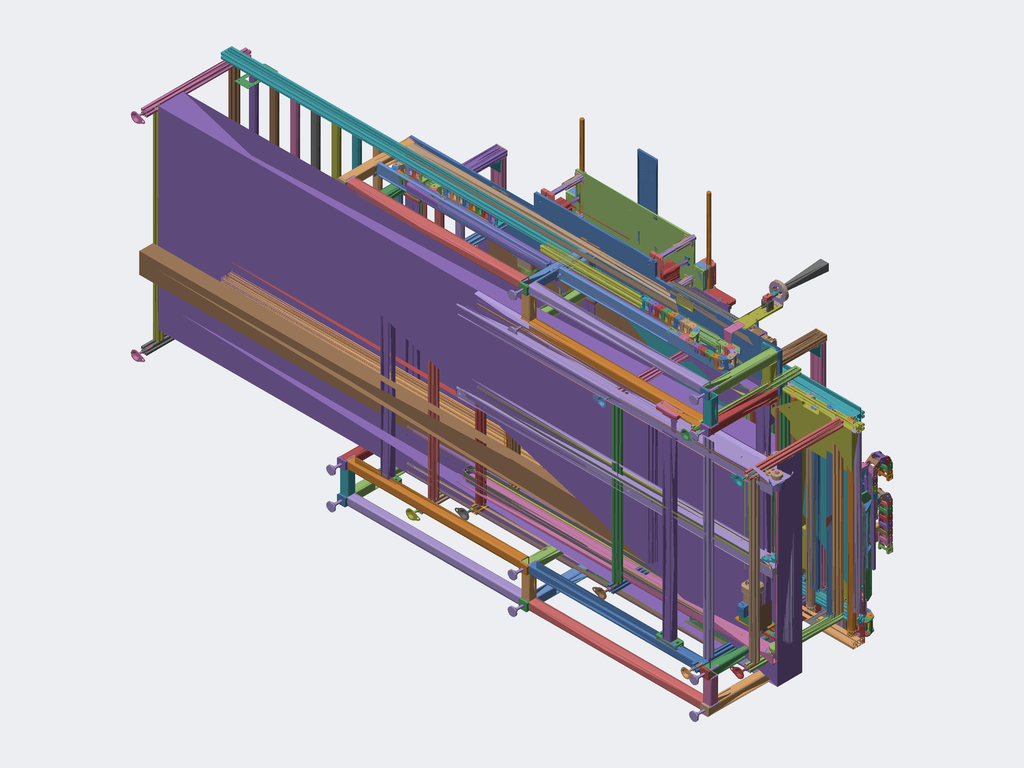Assembly | SolidWorks | 202 different items | 963 placed
Parts list (item | name | quantity | parent item | size | volume | features):
1 | (subassembly) | x2 | in 4 | 57 x 22 x 94 mm | 6979 mm3 | -
2 | (subassembly) | x1 | - | 145.001 x 61.5 x 34.5 mm | 436021 mm3 | -
3 | (subassembly) | x1 | - | 83.2 x 24 x 135 mm | 27538 mm3 | -
4 | (subassembly) | x2 | - | 64 x 60 x 671 mm | 1247970 mm3 | -
5 | (subassembly) | x2 | in 15 | 1463 x 40 x 40 mm | 130548 mm3 | -
6 | (subassembly) | x5 | in 13 | - | 74187256 mm3 | features ReferencePattern 34, LocalLPattern 3
7 | (subassembly) | x21 | in 18 | 95.3 x 80 x 116.633 mm | 320857 mm3 | -
8 | (subassembly) | x2 | - | 223.5 x 705 x 120 mm | 1273117 mm3 | features CompositeCurve 1
9 | (subassembly) | x2 | in 21, 22 | 142.5 x 477.965 x 120 mm | 1151142 mm3 | features ReferencePattern 6, InContextFeatHolder 2, CompositeCurve 1, LocalLPattern 1
10 | (subassembly) | x4 | in 19, 20 | 204 x 77 x 84 mm | 434745 mm3 | -
11 | (subassembly) | x20 | in 14, 16 | 30 x 39 x 30 mm | 17492 mm3 | -
12 | (subassembly) | x1 | - | - | 88653077 mm3 | features ReferencePattern 7, MirrorCompFeat 2, DerivedHolePattern 1
13 | (subassembly) | x1 | - | - | - | features ReferencePattern 40, LocalLPattern 5
14 | (subassembly) | x2 | in 19, 20 | 1270 x 60 x 664 mm | 3435142 mm3 | features ReferencePattern 7, DerivedHolePattern 1, MirrorCompFeat 1
15 | (subassembly) | x2 | - | - | 11809484 mm3 | -
16 | (subassembly) | x2 | in 15 | 190 x 410 x 1645 mm | 3631798 mm3 | features ReferencePattern 6, DerivedHolePattern 1, MirrorCompFeat 1
17 | (subassembly) | x1 | - | - | - | features ReferencePattern 3, CompositeCurve 2, DerivedHolePattern 1
18 | (subassembly) | x7 | in 6, 13 | 1198 x 199.551 x 2300 mm | 9436747 mm3 | features InContextFeatHolder 2, MirrorCompFeat 1, ReferencePattern 1
19 | (subassembly) | x1 | in 12 | - | 39858660 mm3 | features ReferencePattern 11, DerivedHolePattern 2, CompositeCurve 1
20 | (subassembly) | x1 | in 12 | - | 41125199 mm3 | features ReferencePattern 11, DerivedHolePattern 2, CompositeCurve 1
21 | (subassembly) | x1 | in 17 | - | 8582117 mm3 | features ReferencePattern 2, LocalLPattern 1
22 | (subassembly) | x1 | in 17 | - | - | features ReferencePattern 2, CompositeCurve 1, LocalLPattern 1
23 | (subassembly) | x2 | in 17 | 34 x 24 x 680 mm | 137302 mm3 | -
24 | (subassembly) | x2 | in 15 | - | 9829860 mm3 | -
25 | (subassembly) | x2 | in 24 | 123 x 66.8 x 864 mm | 3505638 mm3 | -
26 | (subassembly) | x2 | in 24 | 236 x 83 x 1039 mm | 3946589 mm3 | -
27 | (subassembly) | x2 | in 26 | 172 x 64 x 60 mm | 126138 mm3 | -
28 | Bearing_6004_D42Xd20XT12_Deep Groove Ball Bearing[GBT276-94 | x1 | - | - | - | -
29 | - | x6 | in 8, 9 | 29 x 29.002 x 60.3 mm | 34730 mm3 | features BaseBody 3
30 | - | x7 | in 18 | 282.879 x 60 x 52 mm | 48298 mm3 | features ICE 8, Fillet 3, Extrusion 1, FlatPattern 1, FlattenBends 1, ProcessBends 1, Rip 1, SheetMetal 1, Shell 1
31 | - | x12 | in 6, 13 | 2 x 220 x 100 mm | 34889 mm3 | features ExtruThin 1, Fillet 1, ICE 1
32 | - | x21 | in 7 | 80 x 80 x 50 mm | 223390 mm3 | features ICE 2, CirPattern 1, Extrusion 1, HoleWzd 1, RevCut 1
33 | - | x7 | in 18 | 20 x 20 x 1198 mm | 373288 mm3 | features Extrusion 1, ICE 1
34 | - | x7 | in 18 | 24.001 x 54.65 x 54.65 mm | 18054 mm3 | features BaseBody 1, CirPattern 1, HoleWzd 1
35 | - | x7 | in 18 | 24.001 x 54.65 x 54.65 mm | 19561 mm3 | features BaseBody 1, HoleWzd 1, ICE 1
36 | - | x80 | in 6 | 50 x 50 x 1170 mm | 2265436 mm3 | features HoleWzd 2, ICE 2, Chamfer 1, Extrusion 1, MirrorPattern 1, RevCut 1
37 | - | x6 | in 6, 13 | 43 x 43 x 30 mm | 35397 mm3 | features Extrusion 1, ICE 1
38 | - | x5 | in 6 | 1250 x 740 x 2300 mm | 23808446 mm3 | features ICE 4, Extrusion 1, HoleWzd 1, LPattern 1
39 | - | x2 | in 21, 22 | 630 x 15 x 85 mm | 135946 mm3 | features HoleWzd 3, EdgeFlange 1, Fillet 1, FlatPattern 1, SMBaseFlange 1, SheetMetal 1
40 | - | x8 | in 10 | 40.5 x 5.8 x 4.4 mm | 628.814 mm3 | features BaseBody 1
41 | - | x2 | in 17 | 430 x 20 x 115 mm | 126667 mm3 | features HoleWzd 4, EdgeFlange 1, Fillet 1, FlatPattern 1, SMBaseFlange 1, SheetMetal 1
42 | - | x2 | - | 1259 x 38 x 85 mm | 278401 mm3 | features HoleWzd 4, EdgeFlange 2, Fillet 1, FlatPattern 1, SMBaseFlange 1, SheetMetal 1
43 | - | x4 | in 8, 9 | 100 x 100 x 55 mm | 20982 mm3 | features HoleWzd 3, Fillet 1, FlatPattern 1, SMBaseFlange 1, SheetMetal 1
44 | - | x2 | in 17, 22 | 107.5 x 30 x 55 mm | 14107 mm3 | features HoleWzd 3, Fillet 1, FlatPattern 1, SMBaseFlange 1, SheetMetal 1
45 | - | x6 | in 8, 9 | 125.5 x 22 x 120 mm | 19406 mm3 | features HoleWzd 2, ICE 2, Fillet 1, FlatPattern 1, SMBaseFlange 1, SheetMetal 1
46 | - | x4 | in 9 | 45 x 51 x 60 mm | 15618 mm3 | features ICE 2, ExtruThin 1, Fillet 1, FlatPattern 1, FlattenBends 1, ProcessBends 1, SheetMetal 1
47 | - | x2 | in 15 | 120 x 30 x 360 mm | 79726 mm3 | features ExtruThin 1, Fillet 1, FlatPattern 1, FlattenBends 1, ICE 1, ProcessBends 1, SheetMetal 1
48 | - | x2 | in 15 | 90 x 50 x 80 mm | 23252 mm3 | features ICE 3, ExtruThin 1, Fillet 1
49 | - | x2 | in 9 | 90 x 250 x 5 mm | 108732 mm3 | features ICE 3, Extrusion 1, Fillet 1
50 | - | x4 | in 16 | 190 x 15 x 70 mm | 186782 mm3 | features HoleWzd 4, Chamfer 1, Extrusion 1
51 | - | x12 | in 19, 20 | 60 x 179 x 60 mm | 83421 mm3 | features BaseBody 2
52 | - | x2 | in 16 | 10 x 115 x 370 mm | 331477 mm3 | features HoleWzd 2, Chamfer 1, Extrusion 1, ICE 1
53 | - | x2 | in 16 | 65 x 12 x 370 mm | 282662 mm3 | features HoleWzd 2, Chamfer 1, Extrusion 1, LPattern 1
54 | - | x2 | in 21, 22 | 12 x 105 x 690 mm | 852566 mm3 | features HoleWzd 4, Chamfer 2, Extrusion 1
55 | - | x1 | in 22 | 145 x 12 x 690 mm | 673672 mm3 | features HoleWzd 6, Chamfer 2, Extrusion 1, ICE 1
56 | - | x2 | in 9 | 100 x 148 x 12 mm | 172636 mm3 | features HoleWzd 6, Extrusion 1
57 | - | x2 | in 8 | 80 x 285 x 12 mm | 259377 mm3 | features HoleWzd 5, Chamfer 1, Extrusion 1, ICE 1
58 | - | x4 | in 8, 9 | 50 x 42 x 55 mm | 47186 mm3 | features HoleWzd 2, ICE 2, Chamfer 1, Extrusion 1
59 | - | x1 | in 21 | 145 x 12 x 690 mm | 673672 mm3 | features MirrorStock 1
60 | - | x6 | in 21, 22 | 58 x 10 x 95 mm | 33990 mm3 | features HoleWzd 2, Extrusion 1, ICE 1
61 | - | x4 | in 12 | 130 x 30.7 x 50 mm | 191359 mm3 | features HoleWzd 2, Chamfer 1, Extrusion 1
62 | - | x2 | in 23 | 15 x 12.5 x 680 mm | 106806 mm3 | features ICE 2, BaseBody 1, HoleWzd 1
63 | - | x2 | in 8 | 75 x 10 x 80 mm | 56721 mm3 | features HoleWzd 3, Chamfer 1, Extrusion 1
64 | - | x2 | in 8 | 75 x 10 x 120 mm | 34697 mm3 | features Fillet 2, HoleWzd 2, Extrusion 1, ICE 1
65 | - | x2 | in 21, 22 | 55 x 12 x 148 mm | 94373 mm3 | features HoleWzd 3, Chamfer 1, Extrusion 1
66 | - | x2 | in 21, 22 | 110 x 10 x 105 mm | 47398 mm3 | features Chamfer 1, Extrusion 1, HoleWzd 1, ICE 1, MirrorPattern 1
67 | - | x4 | in 17 | 15 x 13 x 10 mm | 1585 mm3 | features Extrusion 1, HoleWzd 1
68 | - | x4 | in 19, 20 | 310 x 20 x 80 mm | 438735 mm3 | features HoleWzd 4, ICE 2, Chamfer 1, Extrusion 1
69 | - | x4 | in 14 | 15 x 26 x 40 mm | 14020 mm3 | features Chamfer 2, HoleWzd 2, Extrusion 1
70 | - | x2 | in 19, 20 | 1000 x 12 x 320 mm | 3431289 mm3 | features HoleWzd 5, Chamfer 1, Extrusion 1, ICE 1
71 | - | x4 | in 19, 20 | 76 x 41.5 x 130 mm | 406429 mm3 | features Chamfer 1, Extrusion 1, HoleWzd 1
72 | - | x2 | in 14 | 135 x 605 x 12 mm | 965539 mm3 | features HoleWzd 3, Extrusion 1
73 | - | x2 | in 23 | 34 x 19.5 x 57.8 mm | 30496 mm3 | features BaseBody 1
74 | - | x2 | in 14 | 1270 x 60 x 12 mm | 902865 mm3 | features HoleWzd 4, Chamfer 1, Extrusion 1
75 | - | x2 | in 14 | 1270 x 12 x 47 mm | 615944 mm3 | features HoleWzd 4, ICE 2, Chamfer 1, Extrusion 1
76 | - | x8 | in 14 | 25 x 10 x 40 mm | 4716 mm3 | features HoleWzd 2, Chamfer 1, Extrusion 1, ICE 1
77 | - | x2 | in 14 | 1270 x 6 x 15 mm | 113647 mm3 | features Chamfer 1, Extrusion 1, HoleWzd 1
78 | - | x1 | in 20 | 2700 x 15 x 390 mm | 12856560 mm3 | features HoleWzd 7, ICE 4, Chamfer 1, Extrusion 1, Fillet 1, PLine 1
79 | - | x1 | in 19 | 2700 x 15 x 330 mm | 12065498 mm3 | features HoleWzd 7, ICE 4, Chamfer 1, Extrusion 1, Fillet 1, PLine 1
80 | - | x2 | in 16 | 370 x 80 x 1615 mm | 2239494 mm3 | features WeldCornerFeat 2, WeldMemberFeat 2, WeldmentFeature 1
81 | - | x2 | in 19, 20 | 2700 x 516 x 300 mm | 16210960 mm3 | features HoleWzd 9, WeldCornerFeat 6, ICE 4, WeldMemberFeat 3, 3DProfileFeature 1, WeldmentFeature 1
82 | - | x5 | in 12 | 1451 x 150 x 60 mm | 1723034 mm3 | features HoleWzd 2, ICE 1, MirrorSolid 1, WeldMemberFeat 1, WeldmentFeature 1
83 | - | x4 | in 14 | 70 x 70 x 36 mm | 47267 mm3 | features BaseBody 2
84 | - | x1 | in 17 | 129.5 x 557 x 2700 mm | 6948408 mm3 | features HoleWzd 6, ICE 6, Chamfer 3, MirrorSolid 3, WeldMemberFeat 2, MirrorPattern 1, WeldCornerFeat 1, WeldmentFeature 1
85 | - | x4 | in 5 | 66 x 40 x 40 mm | 65274 mm3 | features BaseBody 3
86 | - | x6 | in 8, 9 | 120 x 120 x 20 mm | 177458 mm3 | features Chamfer 1, Extrusion 1, ICE 1
87 | - | x63 | in 7 | 28 x 13 x 13 mm | 1916 mm3 | features BaseBody 1
88 | - | x4 | in 24 | 42.996 x 43 x 52 mm | 57062 mm3 | features BaseBody 1
89 | - | x31 | in 13 | 1380 x 51.459 x 51.986 mm | 596958 mm3 | features ICE 6, BaseBody 1, HoleWzd 1, LPattern 1
90 | - | x1 | in 13 | 1540 x 775 x 4600 mm | 1226148521 mm3 | features ICE 4, BossThin 1, Extrusion 1, LPattern 1
91 | - | x1 | in 13 | 2100 x 85 x 1250 mm | 164068651 mm3 | features ICE 3, BaseBody 1
92 | - | x36 | in 6, 13 | 68 x 121 x 100 mm | 26277 mm3 | features BaseBody 2
93 | - | x1 | - | - | - | features BaseBody 181
94 | - | x2 | in 17 | 912 x 76 x 178.533 mm | 5760586 mm3 | features BaseBody 18, LPattern 1
95 | - | x2 | in 24 | 20 x 20 x 1414 mm | 444221 mm3 | features BaseBody 1, ICE 1
96 | - | x6 | in 8, 9 | 60 x 50 x 350 mm | 603883 mm3 | features Blend 1, Cut 1
97 | - | x6 | in 6, 13 | 60 x 102 x 102.7 mm | 330811 mm3 | features BaseBody 1
98 | - | x7 | in 18 | 189.793 x 59.207 x 17 mm | 45007 mm3 | features ICE 6, Extrusion 1, MirrorPattern 1
99 | - | x4 | in 14 | 25 x 25 x 605 mm | 295385 mm3 | features HoleWzd 2, Chamfer 1, Extrusion 1
100 | - | x8 | in 19, 20 | 30 x 320 x 30 mm | 223294 mm3 | features HoleWzd 2, Chamfer 1, Extrusion 1
101 | - | x7 | in 18 | 72.5 x 159.151 x 2300 mm | 2459772 mm3 | features MirrorStock 1
102 | - | x6 | in 8, 9 | 28 x 34 x 34 mm | 18676 mm3 | features BaseBody 1
103 | - | x1 | in 13 | 57 x 40 x 4600 mm | 1199908 mm3 | features FlatPattern 1, SMBaseFlange 1, SheetMetal 1
104 | - | x21 | in 18 | 2303 x 86 x 50 mm | 856015 mm3 | features ExtruThin 1, Sweep 1
105 | - | x2 | in 21, 22 | 846 x 78 x 155.983 mm | 3838059 mm3 | features BaseBody 19
106 | - | x8 | in 19, 20 | 74 x 74 x 123 mm | 122760 mm3 | features BaseBody 1
107 | - | x4 | in 19, 20 | 76 x 51.5 x 130 mm | 357296 mm3 | features BaseBody 1
108 | - | x13 | in 6, 13, 18 | 273 x 143.386 x 105.972 mm | 1078601 mm3 | features BaseBody 4
109 | - | x16 | in 25, 26 | 24.5 x 15.5 x 50 mm | 13570 mm3 | features BaseBody 1
110 | - | x2 | in 26 | 8.5 x 35.5 x 30 mm | 877.993 mm3 | features BaseBody 1
111 | - | x2 | in 27 | 172 x 64 x 46 mm | 45275 mm3 | features BaseBody 1
112 | - | x2 | in 27 | 172 x 64 x 14 mm | 80863 mm3 | features BaseBody 1
113 | - | x4 | in 25, 26 | 65 x 66.1 x 67 mm | 277180 mm3 | features BaseBody 3
114 | - | x4 | in 24 | 63 x 18.5 x 246 mm | 256185 mm3 | features BaseBody 1
115 | - | x2 | in 25 | 105.5 x 66.1 x 77 mm | 335496 mm3 | features BaseBody 2
116 | - | x2 | in 26 | 142 x 66.1 x 77 mm | 347121 mm3 | features BaseBody 2
117 | - | x4 | in 25, 26 | 65 x 65 x 720 mm | 2838677 mm3 | features BaseBody 1
118 | - | x8 | in 15, 17, 19, 20, 21, 22 | - | - | features RefSurface 65
119 | - | x4 | in 16 | 40 x 5 x 80 mm | 15913 mm3 | features Extrusion 1, Fillet 1
120 | - | x2 | in 26 | - | - | features RefSurface 10
121 | - | x2 | in 4 | 54 x 50 x 604 mm | 1228026 mm3 | features BaseBody 1
122 | - | x2 | in 4 | 32 x 7.6 x 48 mm | 3951 mm3 | features BaseBody 1
123 | - | x2 | in 4 | 53 x 57 x 13 mm | 21853 mm3 | features BaseBody 1
124 | - | x2 | in 4 | 53 x 56.359 x 48 mm | 87261 mm3 | features BaseBody 1
125 | - | x2 | in 1 | 12 x 16.25 x 5.5 mm | 322.658 mm3 | features BaseBody 1
126 | - | x2 | in 4 | 27 x 18 x 18 mm | 1018 mm3 | features BaseBody 1
127 | - | x2 | in 1 | 5.54 x 2 x 5.54 mm | 44.4 mm3 | features BaseBody 1
128 | - | x2 | in 1 | 5.54 x 2 x 5.54 mm | 44.4 mm3 | features BaseBody 1
129 | - | x2 | in 1 | 5.54 x 2 x 5.54 mm | 44.4 mm3 | features BaseBody 1
130 | - | x1 | - | 2060 x 50 x 1250 mm | 5816564 mm3 | features ICE 5, Extrusion 1
131 | - | x2 | in 1 | 5.54 x 2 x 5.54 mm | 44.4 mm3 | features BaseBody 1
132 | - | x2 | in 1 | - | - | features RefSurface 1
133 | - | x2 | in 1 | - | - | features RefSurface 1
134 | - | x2 | in 1 | - | - | features RefSurface 1
135 | - | x2 | in 1 | - | - | features RefSurface 1
136 | - | x2 | in 4 | - | - | features RefSurface 2
137 | - | x2 | in 4 | 54 x 47.5 x 10 mm | 14283 mm3 | features BaseBody 1
138 | - | x2 | in 4 | 13.6 x 15.5 x 27.7 mm | 2180 mm3 | features BaseBody 1
139 | - | x2 | in 4 | 27 x 18 x 18 mm | 1018 mm3 | features BaseBody 1
140 | - | x2 | in 4 | 13.6 x 15.5 x 27.7 mm | 2180 mm3 | features BaseBody 1
141 | - | x6 | in 26 | 26 x 39 x 13.7 mm | 3551 mm3 | features BaseBody 1
142 | - | x2 | in 4 | 13.6 x 15.5 x 27.7 mm | 2180 mm3 | features BaseBody 1
143 | - | x2 | in 4 | 27 x 18 x 18 mm | 1018 mm3 | features BaseBody 1
144 | - | x1 | - | 82 x 66 x 554 mm | 2405342 mm3 | features BaseBody 1
145 | - | x1 | - | 13.6 x 15.5 x 27.7 mm | 2180 mm3 | features BaseBody 1
146 | - | x1 | - | 13.6 x 15.5 x 27.7 mm | 2180 mm3 | features BaseBody 1
147 | - | x1 | - | 27 x 18 x 18 mm | 1018 mm3 | features BaseBody 1
148 | - | x1 | - | 13.6 x 15.5 x 27.7 mm | 2180 mm3 | features BaseBody 1
149 | - | x1 | - | 146 x 62 x 12 mm | 64829 mm3 | features BaseBody 1
150 | - | x1 | - | 140.075 x 56.575 x 22.3 mm | 156798 mm3 | features BaseBody 1
151 | - | x1 | - | - | - | features RefSurface 1
152 | - | x4 | in 16 | 80.8 x 80.8 x 76 mm | 99581 mm3 | features BaseBody 1
153 | - | x1 | - | - | - | features RefSurface 1
154 | - | x1 | - | - | - | features RefSurface 1
155 | - | x1 | - | - | - | features RefSurface 1
156 | - | x1 | - | - | - | features RefSurface 1
157 | - | x1 | - | 5.5 x 5.5 x 3 mm | 63.35 mm3 | features BaseBody 1
158 | - | x1 | - | 5.5 x 5.5 x 3 mm | 63.35 mm3 | features BaseBody 1
159 | - | x1 | - | 5.5 x 5.5 x 3 mm | 63.35 mm3 | features BaseBody 1
160 | - | x1 | - | 5.5 x 5.5 x 3 mm | 63.35 mm3 | features BaseBody 1
161 | - | x1 | - | 145.001 x 61.5 x 34.5 mm | 279097 mm3 | features BaseBody 1
162 | - | x1 | - | - | - | features RefSurface 1
163 | - | x4 | in 16 | 80 x 80 x 30 mm | 51823 mm3 | features BaseBody 1
164 | - | x1 | - | - | - | features RefSurface 1
165 | - | x1 | - | - | - | features RefSurface 1
166 | - | x1 | - | 5.54 x 2 x 5.54 mm | 44.4 mm3 | features BaseBody 1
167 | - | x1 | - | 5.54 x 2 x 5.54 mm | 44.4 mm3 | features BaseBody 1
168 | - | x1 | - | 5.54 x 2 x 5.54 mm | 44.4 mm3 | features BaseBody 1
169 | - | x1 | - | 5.54 x 2 x 5.54 mm | 44.4 mm3 | features BaseBody 1
170 | - | x1 | - | - | - | features RefSurface 1
171 | - | x1 | - | - | - | features RefSurface 1
172 | - | x1 | - | - | - | features RefSurface 1
173 | - | x1 | - | - | - | features RefSurface 1
174 | - | x4 | in 10 | 121 x 84 x 77 mm | 331799 mm3 | features BaseBody 1
175 | - | x1 | - | 80 x 63 x 15 mm | 53710 mm3 | features BaseBody 1
176 | - | x1 | - | 82 x 73.6 x 37.1 mm | 61964 mm3 | features BaseBody 1
177 | - | x1 | - | 4 x 17 x 15 mm | 361.162 mm3 | features BaseBody 1
178 | - | x1 | - | 27 x 18 x 18 mm | 1018 mm3 | features BaseBody 1
179 | - | x1 | - | 27 x 18 x 18 mm | 1018 mm3 | features BaseBody 1
180 | - | x80 | in 6 | 195.3 x 45.3 x 7 mm | 6104 mm3 | features ExtruThin 1
181 | - | x5 | in 6 | 195.3 x 45.3 x 9.4 mm | 8197 mm3 | features ExtruThin 1
182 | - | x20 | in 11 | 30 x 30 x 39 mm | 17492 mm3 | features BaseBody 1, ICE 1
183 | - | x2 | in 26 | 116 x 65 x 65 mm | 248255 mm3 | features BaseBody 3
184 | - | x2 | in 15 | 165 x 64 x 30 mm | 211731 mm3 | features BaseBody 2
185 | - | x4 | in 10 | 121.5 x 62.5 x 62.5 mm | 101686 mm3 | features BaseBody 1
186 | - | x21 | in 7 | 110 x 62 x 33.3 mm | 91720 mm3 | features ICE 2, Extrusion 1
187 | - | x4 | in 24 | 127 x 65 x 38 mm | 109407 mm3 | features BaseBody 1
188 | - | x2 | in 21, 22 | - | 832857 mm3 | features BaseBody 13, LPattern 4
189 | - | x2 | - | - | 907035 mm3 | features BaseBody 13, LPattern 3
190 | - | x2 | in 17 | - | 1022357 mm3 | features BaseBody 13, LPattern 3
191 | - | x4 | in 19, 20 | 36 x 52 x 24 mm | 16208 mm3 | features BaseBody 2, Chamfer 1, ICE 1
192 | - | x6 | in 6, 13 | 90 x 203 x 135 mm | 261739 mm3 | features ICE 2, ExtruThin 1, Fillet 1
193 | - | x7 | in 18 | 72.5 x 159.151 x 2300 mm | 2459772 mm3 | features ICE 6, BossThin 2, Fillet 2, ExtruThin 1, FlatPattern 1, FlattenBends 1, ProcessBends 1, SheetMetal 1
194 | - | x7 | in 18 | 60 x 108 x 2300 mm | 1846867 mm3 | features ICE 6, Fillet 3, BossThin 2, ExtruThin 1, FlatPattern 1, FlattenBends 1, ProcessBends 1, SheetMetal 1
195 | - | x7 | in 18 | 140 x 113 x 190 mm | 218037 mm3 | features ICE 6, Fillet 3, Cut 1, DeleteBody 1, ExtruThin 1, MirrorSolid 1
196 | - | x1 | - | - | - | features RefSurface 137, BaseBody 102
197 | GRH8-L10-400-BL-P40-C4_0 | x1 | - | - | - | -
198 | MKR65-R-X1 (subassembly) | x1 | - | - | - | -
199 | MKR65-X2 (subassembly) | x1 | - | - | - | -
200 | SJCB- 40C- RD_SJCB-40C-16X18 | x1 | - | - | - | -
201 | 同动轴 | x1 | - | - | - | -
202 | 轴承支撑座 | x1 | - | - | - | -
Mates (type | each side: item.copy, entity, surface, feature):
In the top assembly
Coincident | assembly face | assembly face
Slot | assembly face | assembly face | 2 times
Coincident | 77.1 face plane Boss-Extrude 1 | 130.1 face plane Boss-Extrude 1
Coincident | 79.1 face plane 分割线1 | 84.1 face plane Boss-Extrude 2
Concentric | 79.1 face cylinder M8 Tapped Hole 2 | 84.1 face cylinder Ø9.0 (9) DiameterHole 1 | 2 times
Slot | 79.1 face cylinder M5 Tapped Hole 1 | 109.1 face plane 输入1
Coincident | 78.1 face plane 分割线1 | 109.2 face plane 输入1
Slot | 109.3 face cylinder 输入1 | 78.1 face cylinder M5 Tapped Hole 1 | 2 times
Coincident | 78.1 face plane 分割线1 | 109.4 face plane 输入1
Parallel | 78.1 face plane 分割线1 | 57.1 face plane Boss-Extrude 1
Coincident | 78.1 face plane 分割线1 | 121.1 face plane 输入1
Coincident | 63.1 face plane Boss-Extrude 1 | 132.1 face plane 曲Face-输入1
Concentric | 63.1 face cylinder 打Hole尺寸(%根据)内六角圆柱头Screw的类型1 | 132.1 face cylinder 曲Face-输入1 | 2 times
Concentric | 78.1 face cylinder M4 Tapped Hole 2 | 121.1 face cylinder 输入1 | 2 times
Coincident | 78.1 face plane 分割线1 | 121.2 face plane 输入1
Concentric | 78.1 face cylinder M4 Tapped Hole 2 | 121.2 face cylinder 输入1 | 2 times
Coincident | 132.2 face plane 曲Face-输入1 | 63.2 face plane Boss-Extrude 1
Concentric | 132.2 face cylinder 曲Face-输入1 | 63.2 face cylinder 打Hole尺寸(%根据)内六角圆柱头Screw的类型1 | 2 times
Coincident | 42.1 face plane Base-Flange 1 | 189.1 face plane VEP01-F50-002-1-solid1
Concentric | 42.1 face cylinder M4 Tapped Hole 1 | 189.1 face cylinder VEP01-F50-002-1-solid1 | 2 times
Coincident | 81.1 face plane  D:\PROGRAM FILES\SOLIDWORKS CORP\SOLIDWORKS\LANG\CHINESE-SIMPLIFIED\WELDMENT PROFILES\ISO\SQUARE TUBE\60 X 60 X 5 - 丢失(11) | 42.1 face plane Edge-Flange 2
Slot | 81.1 face cylinder M5 Tapped Hole 1 | 42.1 face cylinder M5 间隙槽口1
Coincident | 81.1 plane | 91.1 select_type:25
Width | 90.1 face plane Boss-Extrude 1 | 90.1 face plane Boss-Extrude 1 | 81.2 face plane  D:\PROGRAM FILES\SOLIDWORKS CORP\SOLIDWORKS\LANG\CHINESE-SIMPLIFIED\WELDMENT PROFILES\ISO\SQUARE TUBE\60 X 60 X 5 - 丢失(2) | 81.1 face plane  D:\PROGRAM FILES\SOLIDWORKS CORP\SOLIDWORKS\LANG\CHINESE-SIMPLIFIED\WELDMENT PROFILES\ISO\SQUARE TUBE\60 X 60 X 5 - 丢失(2)
Coincident | 51.1 face plane _WAD36-D60-M16-L150-01-1-solid1 | 92.1 face plane HI_WAN11-D100-M12-L100-001-1-solid1
Coincident | 123.1 face plane 输入1 | 196.1 face plane 31011590_AF0_ASM-1/31091610_AF0_ASM-1/31150289_AF1-1-solid1
Concentric | 123.1 face cylinder 输入1 | 196.1 face cylinder 31041368-ZP_AF0_ASM-1/31071163_AF0-1-solid1
Parallel | 78.1 face plane 分割线1 | 196.1 face plane 31011590_AF0_ASM-1/31091610_AF0_ASM-1/31150289_AF1-1-solid1
Coincident | 90.1 face plane Boss-Extrude 1 | 93.1 face plane 新输送线-1/Profile-1-solid6
Coincident | 90.1 face plane Extrude-薄壁1 | 93.1 face plane 新输送线-1/Profile-1-solid15
Coincident | 91.1 face plane Boss-Extrude 3 | 93.1 face plane 新输送线-1/垫子新-1-solid2
Width | 130.1 face plane Boss-Extrude 1 | 130.1 face plane Boss-Extrude 1 | 93.1 face plane 新输送线-1/垫子新-1-solid2 | 93.1 face plane 新输送线-1/垫子新-1-solid2 | 2 times
Parallel | 79.1 face plane Boss-Extrude 1 | 109.1 face plane 输入1
In subassembly 12
Coincident | 81.3 face plane Boss-Extrude 8 | 82.1 face plane Mirror 1
Slot | 82.1 face cylinder M12 间隙槽口1 | 81.3 face cylinder M12 Tapped Hole 2 | 2 times
Coincident | 81.4 face plane Boss-Extrude 8 | 82.1 face plane Boss-Extrude 1
Coincident | 81.4 face plane  D:\PROGRAM FILES\SOLIDWORKS CORP\SOLIDWORKS\LANG\CHINESE-SIMPLIFIED\WELDMENT PROFILES\ISO\SQUARE TUBE\60 X 60 X 5 - 丢失(11) | 81.3 face plane  D:\PROGRAM FILES\SOLIDWORKS CORP\SOLIDWORKS\LANG\CHINESE-SIMPLIFIED\WELDMENT PROFILES\ISO\SQUARE TUBE\60 X 60 X 5 - 丢失(11)
Coincident | 81.4 face plane Boss-Extrude 1 | 81.3 face plane Boss-Extrude 1
Coincident | 61.1 face plane Boss-Extrude 1 | 82.1 face plane 方管 60 X 60 X 5.0(1)
Concentric | 61.1 face cylinder 打Hole尺寸(%根据)内六角圆柱头Screw的类型1 | 82.1 face cylinder M6 Tapped Hole 1 | 2 times
In subassembly 20
Coincident | 71.1 face plane Boss-Extrude 1 | 70.1 face plane Boss-Extrude 1
Coincident | 71.1 face plane Boss-Extrude 1 | 107.1 face plane 输入1 | 2 times
Coincident | 71.2 face plane Boss-Extrude 1 | 70.1 face plane Boss-Extrude 1
Concentric | 71.2 face cylinder M6 Tapped Hole 1 | 70.1 face cylinder 打Hole尺寸(%根据)内六角圆柱头Screw的类型2 | 2 times
Concentric | 71.1 face cylinder M6 Tapped Hole 1 | 70.1 face cylinder 打Hole尺寸(%根据)内六角圆柱头Screw的类型2 | 2 times
Concentric | 71.1 face cylinder M6 Tapped Hole 1 | 107.1 face cylinder 输入1
Concentric | 71.2 face cylinder M6 Tapped Hole 1 | 107.2 face cylinder 输入1 | 2 times
Coincident | 71.2 face plane Boss-Extrude 1 | 107.2 face plane 输入1
Concentric | 99.1 face cylinder Boss-Extrude 1 | 107.2 face cylinder 输入1
Concentric | 191.1 face cylinder HI_WHD71-M10-1.5-002-1-solid1 | 185.1 face cylinder 输入1
Coincident | 191.1 face plane HI_WHD71-M10-1.5-002-1-solid1 | 185.1 face plane 输入1
Concentric | 191.2 face cylinder HI_WHD71-M10-1.5-002-1-solid1 | 185.2 face cylinder 输入1
Coincident | 191.2 face plane HI_WHD71-M10-1.5-002-1-solid1 | 185.2 face plane 输入1
Coincident | 100.1 face plane Boss-Extrude 1 | 78.2 face plane Cut-Extrude 2
Concentric | 100.1 face cylinder M10 Tapped Hole 1 | 78.2 face cylinder 打Hole尺寸(%根据)内六角圆柱头Screw的类型3
Concentric | 100.1 face cylinder Boss-Extrude 1 | 106.1 face cylinder 输入1
Coincident | 70.1 face plane Boss-Extrude 1 | 106.1 face plane 输入1
Concentric | 70.1 face cylinder Ø25.0 (45.5) DiameterHole 1 | 106.1 face cylinder 输入1
Concentric | 70.1 face cylinder M6 Tapped Hole 2 | 106.1 face cylinder 输入1
Concentric | 70.1 face cylinder M6 Tapped Hole 1 | 191.2 face cylinder HI_WHD71-M10-1.5-001-1-solid1
Concentric | 70.1 face cylinder M6 Tapped Hole 1 | 191.1 face cylinder HI_WHD71-M10-1.5-001-1-solid1
Coincident | 70.1 face plane Boss-Extrude 1 | 191.1 face plane HI_WHD71-M10-1.5-001-1-solid1
Coincident | 78.2 face | 81.5 face plane Boss-Extrude 2
Concentric | 78.2 face cylinder 打Hole尺寸(%根据)内六角圆柱头Screw的类型1 | 81.5 face cylinder M8 Tapped Hole 1 | 2 times
Concentric | 100.2 face cylinder Boss-Extrude 1 | 68.1 face cylinder Cut-Extrude 1
Concentric | 100.3 face cylinder Boss-Extrude 1 | 68.1 face cylinder Cut-Extrude 1
Coincident | 174.1 face plane 输入1 | 68.1 face plane Boss-Extrude 1
Concentric | 174.1 face cylinder 输入1 | 68.1 face cylinder 打Hole尺寸(%根据)内六角圆柱头Screw的类型2 | 2 times
Concentric | 100.4 face cylinder Boss-Extrude 1 | 68.2 face cylinder Cut-Extrude 1
Parallel | 70.1 face plane Boss-Extrude 1 | 81.5 face plane  D:\PROGRAM FILES\SOLIDWORKS CORP\SOLIDWORKS\LANG\CHINESE-SIMPLIFIED\WELDMENT PROFILES\ISO\SQUARE TUBE\60 X 60 X 5 - 丢失(2)
Concentric | 100.1 face cylinder Boss-Extrude 1 | 68.2 face cylinder Cut-Extrude 1
Coincident | 68.1 face plane Boss-Extrude 1 | 68.2 face plane Boss-Extrude 1
Coincident | 174.2 face plane 输入1 | 68.2 face plane Boss-Extrude 1
Concentric | 174.2 face cylinder 输入1 | 68.2 face cylinder 打Hole尺寸(%根据)内六角圆柱头Screw的类型2 | 2 times
Coincident | 70.1 face plane Boss-Extrude 1 | 20.1 face
Concentric | 70.1 face cylinder M5 Tapped Hole 1 | 20.1 face
Concentric | 70.1 face | 20.1 face
Concentric | 81.5 face cylinder M16 Tapped Hole 1 | 51.2 face cylinder _WAD36-D60-M16-L150-01-1-solid1
DistanceDim | 81.5 face plane Boss-Extrude 1 | 51.2 face plane _WAD36-D60-M16-L150-01-1-solid1
Coincident | 20.1 face | 118.1 face plane 曲Face-输入141
Concentric | 20.1 face | 118.1 face cylinder 曲Face-输入139
Parallel | 20.1 face | 118.1 face plane 曲Face-输入141
DistanceDim | 78.2 face plane 分割线1 | 68.1 face plane Boss-Extrude 1
In subassembly 14
Coincident | 72.1 face plane Boss-Extrude 1 | 74.1 face plane Boss-Extrude 1
Coincident | 74.1 face plane Boss-Extrude 1 | 75.1 face plane Boss-Extrude 1
Concentric | 74.1 face cylinder 打Hole尺寸(%根据)内六角圆柱头Screw的类型1 | 75.1 face cylinder M5 Tapped Hole 1 | 2 times
Coincident | 74.1 face plane Boss-Extrude 1 | 83.1 face plane HI_GBJ12-D25-1-1-solid1
Concentric | 74.1 face cylinder M6 Tapped Hole 1 | 83.1 face cylinder HI_GBJ12-D25-1-1-solid1 | 2 times
Concentric | 99.2 face cylinder Boss-Extrude 1 | 83.1 face cylinder HI_GBJ12-D25-1-1-solid1
Coincident | 74.1 face plane Boss-Extrude 1 | 83.2 face plane HI_GBJ12-D25-1-1-solid1
Concentric | 74.1 face cylinder M6 Tapped Hole 1 | 83.2 face cylinder HI_GBJ12-D25-1-1-solid1 | 2 times
Concentric | 99.3 face cylinder Boss-Extrude 1 | 83.2 face cylinder HI_GBJ12-D25-1-1-solid1
Coincident | 74.1 face plane Boss-Extrude 1 | 99.3 face plane Boss-Extrude 1
Coincident | 99.2 face plane Boss-Extrude 1 | 74.1 face plane Boss-Extrude 1
Concentric | 74.1 face cylinder M4 Tapped Hole 1 | 76.1 face cylinder 打Hole尺寸(%根据)内六角圆柱头Screw的类型1
Concentric | 75.1 face cylinder M4 Tapped Hole 1 | 76.1 face cylinder M4 间隙Hole 1
Coincident | 75.1 face plane Cut-Extrude 1 | 77.2 face plane Boss-Extrude 1
Concentric | 74.1 face cylinder M4 Tapped Hole 1 | 76.2 face cylinder 打Hole尺寸(%根据)内六角圆柱头Screw的类型1
Concentric | 75.1 face cylinder M4 Tapped Hole 1 | 76.2 face cylinder M4 间隙Hole 1
Concentric | 72.1 face cylinder M6 Tapped Hole 1 | 74.1 face cylinder 打Hole尺寸(%根据)内六角圆柱头Screw的类型2
Concentric | 69.1 face cylinder M6 Tapped Hole 2 | 74.1 face cylinder 打Hole尺寸(%根据)内六角圆柱头Screw的类型2
Concentric | 72.1 face cylinder 打Hole尺寸(%根据)内六角圆柱头Screw的类型2 | 69.1 face cylinder M6 Tapped Hole 1
Concentric | 72.1 face cylinder 打Hole尺寸(%根据)内六角圆柱头Screw的类型2 | 69.2 face cylinder M6 Tapped Hole 1
Concentric | 69.2 face cylinder M6 Tapped Hole 2 | 74.1 face cylinder 打Hole尺寸(%根据)内六角圆柱头Screw的类型2
Coincident | 99.3 face plane Boss-Extrude 1 | assembly face
Concentric | 99.3 face cylinder M8 Tapped Hole 1 | assembly face
Concentric | 99.2 face cylinder M8 Tapped Hole 1 | assembly face
Coincident | 75.1 face plane Cut-Extrude 2 | 14.1 face
Concentric | 75.1 face cylinder Cut-Extrude 2 | 14.1 face
Concentric | 75.1 face cylinder M3 Tapped Hole 1 | 77.2 face cylinder 打Hole尺寸(%根据)内六角圆柱头Screw的类型1 | 2 times
In subassembly 10
LimitDistanceDim | 185.3 face plane 输入1 | 174.3 face plane 输入1
Concentric | 174.3 face cylinder 输入1 | 185.3 face cylinder 输入1
In subassembly 19
Coincident | 71.1 face plane Boss-Extrude 1 | 70.1 face plane Boss-Extrude 1
Coincident | 71.1 face plane Boss-Extrude 1 | 107.1 face plane 输入1 | 2 times
Coincident | 71.2 face plane Boss-Extrude 1 | 70.1 face plane Boss-Extrude 1
Concentric | 71.2 face cylinder M6 Tapped Hole 1 | 70.1 face cylinder 打Hole尺寸(%根据)内六角圆柱头Screw的类型2 | 2 times
Concentric | 71.1 face cylinder M6 Tapped Hole 1 | 70.1 face cylinder 打Hole尺寸(%根据)内六角圆柱头Screw的类型2 | 2 times
Concentric | 71.1 face cylinder M6 Tapped Hole 1 | 107.1 face cylinder 输入1
Concentric | 71.2 face cylinder M6 Tapped Hole 1 | 107.2 face cylinder 输入1 | 2 times
Coincident | 71.2 face plane Boss-Extrude 1 | 107.2 face plane 输入1
Concentric | 99.1 face cylinder Boss-Extrude 1 | 107.2 face cylinder 输入1
DistanceDim | 79.2 face plane 分割线1 | 174.1 face plane 输入1
Concentric | 191.1 face cylinder HI_WHD71-M10-1.5-002-1-solid1 | 185.1 face cylinder 输入1
Coincident | 191.1 face plane HI_WHD71-M10-1.5-002-1-solid1 | 185.1 face plane 输入1
Concentric | 191.2 face cylinder HI_WHD71-M10-1.5-002-1-solid1 | 185.2 face cylinder 输入1
Coincident | 191.2 face plane HI_WHD71-M10-1.5-002-1-solid1 | 185.2 face plane 输入1
Coincident | 100.1 face plane Boss-Extrude 1 | 79.2 face plane Cut-Extrude 2
Concentric | 100.1 face cylinder M10 Tapped Hole 1 | 79.2 face cylinder 打Hole尺寸(%根据)内六角圆柱头Screw的类型3
Concentric | 100.1 face cylinder Boss-Extrude 1 | 106.1 face cylinder 输入1
Coincident | 70.1 face plane Boss-Extrude 1 | 106.1 face plane 输入1
Concentric | 70.1 face cylinder Ø25.0 (45.5) DiameterHole 1 | 106.1 face cylinder 输入1
Concentric | 70.1 face cylinder M6 Tapped Hole 2 | 106.1 face cylinder 输入1
Concentric | 70.1 face cylinder M6 Tapped Hole 1 | 191.2 face cylinder HI_WHD71-M10-1.5-001-1-solid1
Concentric | 70.1 face cylinder M6 Tapped Hole 1 | 191.1 face cylinder HI_WHD71-M10-1.5-001-1-solid1
Coincident | 70.1 face plane Boss-Extrude 1 | 191.1 face plane HI_WHD71-M10-1.5-001-1-solid1
Coincident | 79.2 face | 81.5 face plane Boss-Extrude 2
Concentric | 79.2 face cylinder 打Hole尺寸(%根据)内六角圆柱头Screw的类型1 | 81.5 face cylinder M8 Tapped Hole 1 | 2 times
Concentric | 100.2 face cylinder Boss-Extrude 1 | 68.1 face cylinder Cut-Extrude 1
Concentric | 100.3 face cylinder Boss-Extrude 1 | 68.1 face cylinder Cut-Extrude 1
Coincident | 174.1 face plane 输入1 | 68.1 face plane Boss-Extrude 1
Concentric | 174.1 face cylinder 输入1 | 68.1 face cylinder 打Hole尺寸(%根据)内六角圆柱头Screw的类型2 | 2 times
Concentric | 100.4 face cylinder Boss-Extrude 1 | 68.2 face cylinder Cut-Extrude 1
Parallel | 70.1 face plane Boss-Extrude 1 | 81.5 face plane  D:\PROGRAM FILES\SOLIDWORKS CORP\SOLIDWORKS\LANG\CHINESE-SIMPLIFIED\WELDMENT PROFILES\ISO\SQUARE TUBE\60 X 60 X 5 - 丢失(2)
Concentric | 100.1 face cylinder Boss-Extrude 1 | 68.2 face cylinder Cut-Extrude 1
Coincident | 68.1 face plane Boss-Extrude 1 | 68.2 face plane Boss-Extrude 1
Coincident | 174.2 face plane 输入1 | 68.2 face plane Boss-Extrude 1
Concentric | 174.2 face cylinder 输入1 | 68.2 face cylinder 打Hole尺寸(%根据)内六角圆柱头Screw的类型2 | 2 times
Coincident | 70.1 face plane Boss-Extrude 1 | 19.1 face
Concentric | 70.1 face cylinder M5 Tapped Hole 1 | 19.1 face
Concentric | 70.1 face | 19.1 face
Concentric | 118.1 face cylinder 曲Face-输入139 | 19.1 face
Coincident | 118.1 face plane 曲Face-输入141 | 19.1 face
Parallel | 118.1 face plane 曲Face-输入141 | 19.1 face
Concentric | 81.5 face cylinder M16 Tapped Hole 1 | 51.2 face cylinder _WAD36-D60-M16-L150-01-1-solid1
DistanceDim | 81.5 face plane Boss-Extrude 1 | 51.2 face plane _WAD36-D60-M16-L150-01-1-solid1
In subassembly 15
Coincident | 50.1 face plane Boss-Extrude 1 | 114.1 face plane 输入1
Slot | 50.1 face cylinder 打Hole尺寸(%根据)内六角圆柱头Screw的类型5 | 114.1 face cylinder 输入1
Slot | 50.2 face cylinder 打Hole尺寸(%根据)内六角圆柱头Screw的类型5 | 114.2 face cylinder 输入1
Concentric | 118.1 face cylinder 曲Face-输入139 | 15.1 face
Coincident | 118.1 face plane 曲Face-输入141 | 15.1 face
Parallel | 118.1 face plane 曲Face-输入141 | 15.1 face
Concentric | 118.1 face cylinder 曲Face-输入139 | 183.1 face cylinder 输入2
Parallel | 118.1 face plane 曲Face-输入141 | 183.1 face plane 输入3
Coincident | 118.1 face plane 曲Face-输入141 | 183.1 face plane 输入3
Coincident | 113.1 face plane 输入1 | 15.1 face
Coincident | 117.1 face plane 输入1 | 15.1 edge
Coincident | 184.1 face plane _TCL-16x100-0_100fp-1-solid1 | 47.1 face plane Extrude-薄壁1
Concentric | 184.1 face cylinder _TCL-16x100-0_100fp-1-solid1 | 47.1 face cylinder Cut-Extrude 1 | 2 times
DistanceDim | 47.1 face plane Extrude-薄壁1 | 80.1 face plane Aluminium Profile 40 X 80W X R4.5(1)
DistanceDim | 80.1 face plane Aluminium Profile 40 X 80W X R4.5(1) | 184.1 face plane _TC-L-16x100100_b-1-solid1
Coincident | 184.1 face plane _TC-L-16x100100_b-1-solid1 | 48.1 face plane Extrude-薄壁1
Coincident | 80.1 face plane Aluminium Profile 40 X 80W X R4.5(1) | 48.1 face plane Extrude-薄壁1
In subassembly 5
Coincident | 5.1 face | 85.1 face plane _DCJ01-D40-B-d16-e16-003-1-solid1
Concentric | 5.1 face | 85.2 face cylinder _DCJ01-D40-B-d16-e16-001-1-solid1
Coincident | 5.1 face | 85.2 face plane _DCJ01-D40-B-d16-e16-001-1-solid1
Concentric | 5.1 face | 85.1 face cylinder _DCJ01-D40-B-d16-e16-003-1-solid1
In subassembly 16
Coincident | 53.1 face plane Boss-Extrude 1 | 52.1 face plane Boss-Extrude 1
Concentric | 53.1 face | 16.1 face
Concentric | 52.1 face cylinder M4 Tapped Hole 1 | 53.1 face cylinder 打Hole尺寸(%根据)内六角圆柱头Screw的类型1 | 2 times
Concentric | 50.3 face cylinder 打Hole尺寸(%根据)内六角圆柱头Screw的类型3 | 80.2 face cylinder Aluminium Profile 40 X 80W X R4.5(7) | 2 times
Coincident | 80.2 face plane Aluminium Profile 40 X 80W X R4.5(1) | 52.1 face plane Boss-Extrude 1
DistanceDim | 80.2 face plane Aluminium Profile 40 X 80W X R4.5(1) | 52.1 face plane Boss-Extrude 1
Coincident | 80.2 plane | 52.1 plane
Coincident | 80.2 face plane Aluminium Profile 40 X 80W X R4.5(7) | 50.4 face plane Boss-Extrude 1
Coincident | 50.3 face plane Boss-Extrude 1 | 80.2 face plane Aluminium Profile 40 X 80W X R4.5(7)
Coincident | 80.2 face plane Aluminium Profile 40 X 80W X R4.5(1) | 152.1 face plane 输入1
Coincident | 80.2 face plane Aluminium Profile 40 X 80W X R4.5(7) | 152.1 face plane 输入1
Width | 152.1 face plane 输入1 | 152.1 face plane 输入1 | 80.2 face plane Aluminium Profile 40 X 80W X R4.5(1) | 80.2 face plane Aluminium Profile 40 X 80W X R4.5(1)
Coincident | 80.2 face plane 剪裁/延伸2 | 119.1 face plane Boss-Extrude 1
Coincident | 80.2 face plane Aluminium Profile 40 X 80W X R4.5(7) | 119.1 face plane Boss-Extrude 1 | 2 times
Coincident | 16.1 face | 53.1 face
Concentric | 80.2 face cylinder Aluminium Profile 40 X 80W X R4.5(7) | 50.4 face cylinder 打Hole尺寸(%根据)内六角圆柱头Screw的类型3 | 2 times
Coincident | 50.4 face plane Boss-Extrude 1 | 163.1 face plane ABC01-4010-80B-30_001-1-solid1
Coincident | 80.2 face plane Aluminium Profile 40 X 80W X R4.5(7) | 163.1 face plane ABC01-4010-80B-30_001-1-solid1
Width | 163.1 face plane ABC01-4010-80B-30_001-1-solid1 | 163.1 face plane ABC01-4010-80B-30_001-1-solid1 | 50.4 face plane Boss-Extrude 1 | 50.4 face plane Boss-Extrude 1
In subassembly 24
DistanceDim | 114.3 face plane 输入1 | 109.5 face plane 输入1
DistanceDim | 114.3 face plane 输入1 | 117.2 face plane 输入1
LimitDistanceDim | 116.1 face plane 输入1 | 114.3 face plane 输入1
DistanceDim | 114.4 face plane 输入1 | 117.3 face plane 输入1
Coincident | 114.3 face plane 输入1 | 114.4 face plane 输入1 | 2 times
Coincident | 109.5 face plane 输入1 | 109.6 face plane 输入1 | 2 times
DistanceDim | 109.6 face plane 输入1 | 109.5 face plane 输入1
Concentric | 115.1 face cylinder 输入2 | 95.1 face cylinder 输入1
Width | 95.1 face plane Cut-Extrude 1 | 95.1 face plane 输入1 | 115.1 face plane 输入2 | 116.1 face plane 输入1
Width | 88.1 face plane 输入1 | 88.1 face plane 输入1 | 115.1 face plane 输入2 | 95.1 face plane 输入1
Concentric | 88.1 face cylinder 输入1 | 95.1 face cylinder 输入1
Concentric | 95.1 face cylinder 输入1 | 187.1 face cylinder 输入1
Concentric | 95.1 face cylinder 输入1 | 187.2 face cylinder 输入1
Coincident | 187.2 face plane 输入1 | 187.1 face plane 输入1
Parallel | 116.1 face plane 输入1 | 187.2 face plane 输入1
DistanceDim | 187.2 face plane 输入1 | 187.1 face plane 输入1
Width | 187.1 face plane 输入1 | 187.2 face plane 输入1 | 109.7 face plane 输入1 | 109.5 face plane 输入1
In subassembly 8
Concentric | 57.2 face cylinder M5 Tapped Hole 1 | 43.1 face cylinder M5 间隙Hole 1 | 2 times
Coincident | 58.1 face plane Boss-Extrude 1 | 57.2 face plane Cut-Extrude 2
Coincident | 102.1 face plane 输入1 | 96.1 face plane 放样1
Concentric | 96.1 face cylinder Cut-Extrude 1 | 102.1 face cylinder 输入1
Concentric | 102.1 face cylinder 输入1 | 86.1 face cylinder Boss-Extrude 1
Coincident | 102.1 face plane 输入1 | 29.1 face plane 输入3
Concentric | 58.1 face cylinder M3 间隙Hole 1 | 29.1 face cylinder 输入3 | 2 times
Coincident | 58.1 face plane Cut-Extrude 2 | 29.1 face plane 输入3
Coincident | 86.1 face plane Boss-Extrude 1 | 45.1 face plane Base-Flange 1
Coincident | 57.2 face plane Boss-Extrude 1 | 45.1 face plane Base-Flange 1
Concentric | 57.2 face cylinder M5 Tapped Hole 2 | 45.1 face cylinder M5 间隙Hole 1 | 2 times
Concentric | 102.1 face cylinder 输入1 | 29.1 face cone 输入3
Concentric | 86.1 face cylinder Cut-Extrude 1 | 45.1 face cylinder M3 间隙Hole 1
Slot | 58.1 face plane 打Hole尺寸(%根据)内六角圆柱头Screw的类型5 | 57.2 face cylinder M4 Tapped Hole 1
Slot | 58.1 face cylinder 打Hole尺寸(%根据)内六角圆柱头Screw的类型5 | 57.2 face cylinder M4 Tapped Hole 1
Coincident | 57.2 face plane Boss-Extrude 1 | 63.3 face plane Boss-Extrude 1
Concentric | 57.2 face cylinder 打Hole尺寸(%根据)内六角圆柱头Screw的类型1 | 63.3 face cylinder M5 Tapped Hole 1 | 2 times
Concentric | 63.3 face cylinder 打Hole尺寸(%根据)内六角圆柱头Screw的类型2 | 64.1 face cylinder M4 Tapped Hole 1
Concentric | 57.2 face cylinder 打Hole尺寸(%根据)内六角圆柱头Screw的类型2 | 64.1 face cylinder M4 Tapped Hole 2
Coincident | 57.2 face plane Boss-Extrude 1 | 43.1 face plane Base-Flange 1
In subassembly 17
Coincident | 41.1 face plane Base-Flange 1 | 190.1 face plane VEP01-F75-002-1-solid1
Concentric | 41.1 face cylinder M4 Tapped Hole 2 | 190.1 face cylinder VEP01-F75-002-1-solid1 | 2 times
Concentric | 84.2 face cylinder M5 Tapped Hole 1 | 41.1 face cylinder M5 间隙Hole 1 | 2 times
Coincident | 84.2 face plane Boss-Extrude 1 | 41.1 face plane Edge-Flange 1
Coincident | 59.1 face plane | 44.1 face plane Base-Flange 1
Concentric | 59.1 face cylinder | 44.1 face cylinder M5 间隙Hole 1 | 2 times
Coincident | 41.2 face plane Base-Flange 1 | 190.2 face plane VEP01-F75-002-1-solid1
Concentric | 41.2 face cylinder M4 Tapped Hole 2 | 190.2 face cylinder VEP01-F75-002-1-solid1 | 2 times
Coincident | 84.2 face plane Mirror 3 | 41.2 face plane Edge-Flange 1
Concentric | 84.2 face cylinder Mirror 3 | 41.2 face cylinder M5 间隙Hole 1 | 2 times
Concentric | 84.2 face cylinder M4 Tapped Hole 3 | 62.1 face cylinder 打Hole尺寸(%根据)内六角圆柱头Screw的类型1 | 2 times
Concentric | 65.1 face cylinder 打Hole尺寸(%根据)内六角圆柱头Screw的类型1 | 73.1 face cylinder 输入1
Concentric | 84.2 face cylinder M4 Tapped Hole 3 | 62.2 face cylinder 打Hole尺寸(%根据)内六角圆柱头Screw的类型1 | 2 times
Concentric | 65.2 face cylinder 打Hole尺寸(%根据)内六角圆柱头Screw的类型1 | 73.2 face cylinder 输入1
Concentric | 84.2 face cylinder M4 Tapped Hole 4 | 67.1 face cylinder 打Hole尺寸(%根据)内六角圆柱头Screw的类型1
Coincident | 84.2 face plane Boss-Extrude 3 | 67.1 face plane Boss-Extrude 1 | 2 times
Coincident | 84.2 face plane Boss-Extrude 3 | 62.1 face plane 输入1
Coincident | 84.2 face plane Boss-Extrude 3 | 62.2 face plane 输入1
Coincident | 84.2 face plane Mirror 3 | 94.1 face plane _GRH12-L5-500-BC-M-C4(0)body-1-solid1
Concentric | 84.2 face cylinder Mirror 3 | 94.1 face cylinder _GRH12-L5-500-BC-M-C4(0)body-1-solid1
Parallel | 84.2 face plane Mirror 3 | 94.1 face plane _GRH12-L5-500-BC-M-C4(0)body-1-solid1
Coincident | 84.2 face plane Boss-Extrude 1 | 94.2 face plane _GRH12-L5-500-BC-M-C4(0)body-1-solid1
Concentric | 84.2 face cylinder M6 Tapped Hole 1 | 94.2 face cylinder _GRH12-L5-500-BC-M-C4(0)body-1-solid1 | 2 times
In subassembly 22
Coincident | 54.1 face plane Boss-Extrude 1 | 55.1 face plane Boss-Extrude 1
Concentric | 54.1 face cylinder M6 Tapped Hole 1 | 55.1 face cylinder 打Hole尺寸(%根据)内六角圆柱头Screw的类型2 | 2 times
Concentric | 55.1 face cylinder 打Hole尺寸(%根据)内六角圆柱头Screw的类型3 | 60.1 face cylinder M5 Tapped Hole 2
Concentric | 54.1 face cylinder 打Hole尺寸(%根据)内六角圆柱头Screw的类型1 | 60.1 face cylinder M5 Tapped Hole 1
Coincident | 54.1 face plane Boss-Extrude 1 | 39.1 face plane Base-Flange 1
Coincident | 39.1 face plane Base-Flange 1 | 188.1 face plane VEP01-F50-002-1-solid1
Coincident | 55.1 face plane Boss-Extrude 1 | 44.1 face plane Base-Flange 1
Concentric | 55.1 face cylinder M5 Tapped Hole 1 | 44.1 face cylinder M5 间隙Hole 1 | 2 times
Concentric | 39.1 face cylinder M4 Tapped Hole 1 | 188.1 face cylinder LPattern 5 | 2 times
Concentric | 55.1 face cylinder 打Hole尺寸(%根据)内六角圆柱头Screw的类型4 | 65.3 face cylinder M6 Tapped Hole 1 | 2 times
Coincident | 55.1 face plane Boss-Extrude 1 | 65.3 face plane Boss-Extrude 1
Concentric | 65.3 face cylinder 打Hole尺寸(%根据)内六角圆柱头Screw的类型2 | 66.1 face cylinder M5 Tapped Hole 1
Concentric | 55.1 face cylinder 打Hole尺寸(%根据)内六角圆柱头Screw的类型5 | 66.1 face cylinder Mirror 1
Concentric | 54.1 face cylinder M3 Tapped Hole 2 | 39.1 face cone 打Hole尺寸(%根据)开槽沉头木Screw的类型2 | 2 times
Coincident | 54.1 face plane Boss-Extrude 1 | 105.1 face plane _GRH8-L5-450-BC-M-C4(0)body-1-solid1
Concentric | 105.1 face cylinder _GRH8-L5-450-BC-M-C4(0)body-1-solid1 | 54.1 face cylinder M5 Tapped Hole 1
Parallel | 54.1 face plane Boss-Extrude 1 | 105.1 face plane _GRH8-BC-M10_body6-1-solid1
Concentric | 56.1 face cylinder 打Hole尺寸(%根据)内六角圆柱头Screw的类型0 | 105.1 face cylinder _GRH8-450-BC_slider-1-solid1 | 2 times
Coincident | 56.1 face plane Boss-Extrude 1 | 105.1 face plane _GRH8-450-BC_slider-1-solid1
In subassembly 9
Coincident | 56.2 face plane Boss-Extrude 1 | 43.1 face plane Base-Flange 1
Concentric | 56.2 face cylinder M5 Tapped Hole 1 | 43.1 face cylinder M5 间隙Hole 1 | 2 times
Coincident | 102.1 face plane 输入1 | 96.1 face plane 放样1
Concentric | 96.1 face cylinder Cut-Extrude 1 | 102.1 face cylinder 输入1
Concentric | 102.1 face cylinder 输入1 | 86.1 face cylinder Boss-Extrude 1
Coincident | 102.1 face plane 输入1 | 29.1 face plane 输入3
Concentric | 58.1 face cylinder M3 间隙Hole 1 | 29.1 face cylinder 输入3 | 2 times
Coincident | 58.1 face plane Cut-Extrude 2 | 29.1 face plane 输入3
Coincident | 86.1 face plane Boss-Extrude 1 | 45.1 face plane Base-Flange 1
Coincident | 56.2 face plane Boss-Extrude 1 | 45.1 face plane Base-Flange 1
Concentric | 56.2 face cylinder M5 Tapped Hole 2 | 45.1 face cylinder M5 间隙Hole 1 | 2 times
Concentric | 102.1 face cylinder 输入1 | 29.1 face cone 输入3
Concentric | 86.1 face cylinder Cut-Extrude 1 | 45.1 face cylinder M3 间隙Hole 1
Coincident | 29.1 face plane 输入3 | 46.1 face plane Extrude-薄壁1
Concentric | 29.1 face cylinder 输入3 | 46.1 face cylinder Cut-Extrude 1
Parallel | 29.1 face plane 输入3 | 46.1 face plane Extrude-薄壁1
Coincident | 56.2 face plane Boss-Extrude 1 | 49.1 face plane Boss-Extrude 1
Width | 49.1 face plane Boss-Extrude 1 | 49.1 face plane Boss-Extrude 1 | 56.2 face plane Boss-Extrude 1 | 56.2 face plane Boss-Extrude 1
In subassembly 23
DistanceDim | 73.3 face plane 输入1 | 62.3 face plane 输入1
Width | 73.3 face plane 输入1 | 73.3 face plane 输入1 | 62.3 face plane 输入1 | 62.3 face plane 输入1
In subassembly 21
Coincident | 54.1 face plane Boss-Extrude 1 | 39.1 face plane Base-Flange 1
Coincident | 54.1 face plane Boss-Extrude 1 | 59.2 face plane
Concentric | 54.1 face cylinder M6 Tapped Hole 1 | 59.2 face cylinder | 2 times
Concentric | 59.2 face cylinder | 60.1 face cylinder M5 Tapped Hole 2
Concentric | 54.1 face cylinder 打Hole尺寸(%根据)内六角圆柱头Screw的类型1 | 60.1 face cylinder M5 Tapped Hole 1
Coincident | 39.1 face plane Base-Flange 1 | 188.1 face plane VEP01-F50-002-1-solid1
Concentric | 39.1 face cylinder M4 Tapped Hole 1 | 188.1 face cylinder LPattern 5 | 2 times
Concentric | 54.1 face cylinder M3 Tapped Hole 2 | 39.1 face cone 打Hole尺寸(%根据)开槽沉头木Screw的类型2 | 2 times
Coincident | 59.2 face plane | 65.3 face plane Boss-Extrude 1
Concentric | 59.2 face cylinder | 65.3 face cylinder M6 Tapped Hole 1 | 2 times
Concentric | 65.3 face cylinder 打Hole尺寸(%根据)内六角圆柱头Screw的类型2 | 66.1 face cylinder Mirror 1
Concentric | 59.2 face cylinder | 66.1 face cylinder M5 Tapped Hole 1
Coincident | 54.1 face plane Boss-Extrude 1 | 105.1 face plane _GRH8-L5-450-BC-M-C4(0)body-1-solid1
Concentric | 54.1 face cylinder M5 Tapped Hole 1 | 105.1 face cylinder _GRH8-L5-450-BC-M-C4(0)body-1-solid1
Concentric | 56.1 face cylinder 打Hole尺寸(%根据)内六角圆柱头Screw的类型0 | 105.1 face cylinder _GRH8-450-BC_slider-1-solid1 | 2 times
Parallel | 54.1 face plane Boss-Extrude 1 | 105.1 face plane _GRH8-BC-M10_body6-1-solid1
In subassembly 13
Concentric | 37.1 face cylinder Boss-Extrude 1 | 192.1 face cylinder Cut-Extrude 1
Concentric | 37.1 face cylinder Cut-Extrude 1 | 108.1 face cylinder 100GF-H-18-1-solid1
Coincident | 192.1 face plane Extrude-薄壁1 | 108.1 face plane 100GF-H-18-1-solid2
Coincident | 31.1 face plane Extrude-薄壁1 | 97.1 face plane 输入1
Concentric | 31.1 face cylinder Cut-Extrude 1 | 97.1 face cylinder 输入1 | 2 times
Coincident | 90.2 face plane Boss-Extrude 1 | 89.1 face plane Boss-Extrude 2
Concentric | 90.2 face cylinder Cut-Extrude 1 | 89.1 face cylinder Boss-Extrude 2
Coincident | 90.2 face plane Boss-Extrude 2 | 193.1 face plane Extrude-薄壁1
Concentric | 90.2 face cylinder Boss-Extrude 3 | 92.2 face cylinder HI_WAN11-D100-M12-L100-001-1-solid1
DistanceDim | 92.2 face plane HI_WAN11-D100-M12-L100-001-1-solid1 | 90.2 face plane Boss-Extrude 1
DistanceDim | 90.2 face plane Boss-Extrude 1 | 91.2 face plane 输入1
Coincident | 92.3 face plane HI_WAN11-D100-M12-L100-001-1-solid1 | 92.4 face plane HI_WAN11-D100-M12-L100-001-1-solid1
Coincident | 90.2 face plane Boss-Extrude 1 | 38.1 face plane Boss-Extrude 1
Coincident | 90.2 face plane Boss-Extrude 1 | 103.1 face plane Base-Flange 1 | 3 times
Width | 91.2 face plane 输入1 | 91.2 face plane 输入1 | 38.1 face plane Boss-Extrude 1 | 90.2 face plane Boss-Extrude 1
In subassembly 6
Coincident | 38.2 face plane Boss-Extrude 1 | 36.1 face plane Boss-Extrude 1
Concentric | 38.2 face cylinder 打Hole尺寸(%根据)内六角圆柱头Screw的类型1 | 36.1 face cylinder M8 Tapped Hole 1
DistanceDim | 193.1 face plane Extrude-薄壁1 | 38.2 face plane Boss-Extrude 2
Concentric | 38.2 face cylinder Boss-Extrude 2 | 92.2 face cylinder HI_WAN11-D100-M12-L100-001-1-solid1
DistanceDim | 92.2 face plane HI_WAN11-D100-M12-L100-001-1-solid1 | 38.2 face plane Boss-Extrude 1
DistanceDim | 38.2 face plane Boss-Extrude 1 | 192.1 face plane Extrude-薄壁1
Coincident | 38.2 face plane Boss-Extrude 1 | 192.1 face plane Extrude-薄壁1
Coincident | 36.1 face plane Cut-Extrude 2 | 180.1 face plane Extrude-薄壁1
Concentric | 36.1 face cylinder Boss-Extrude 1 | 180.1 face cylinder Extrude-薄壁1
Concentric | 36.2 face cylinder Boss-Extrude 1 | 180.2 face cylinder Extrude-薄壁1
Concentric | 36.3 face cylinder Boss-Extrude 1 | 180.2 face cylinder Extrude-薄壁1
Concentric | 37.1 face cylinder Boss-Extrude 1 | 181.1 face cylinder Extrude-薄壁1
Concentric | 36.4 face cylinder Boss-Extrude 1 | 181.1 face cylinder Extrude-薄壁1
Concentric | 37.1 face cylinder Boss-Extrude 1 | 192.1 face cylinder Cut-Extrude 1
Coincident | 38.2 face plane Boss-Extrude 1 | 101.1 face plane
Concentric | 37.1 face cylinder Cut-Extrude 1 | 108.1 face cylinder 100GF-H-18-1-solid1
Coincident | 192.1 face plane Extrude-薄壁1 | 108.1 face plane 100GF-H-18-1-solid2
Coincident | 38.2 face plane Boss-Extrude 1 | 31.1 face plane Extrude-薄壁1
Coincident | 31.1 face plane Extrude-薄壁1 | 97.1 face plane 输入1
Concentric | 31.1 face cylinder Cut-Extrude 1 | 97.1 face cylinder 输入1 | 2 times
Coincident | 38.2 face plane Boss-Extrude 2 | 31.2 face plane Extrude-薄壁1
Coincident | 38.2 face plane Boss-Extrude 3 | 194.1 face plane Extrude-薄壁1
In subassembly 18
Concentric | 33.1 face cylinder Boss-Extrude 1 | 34.1 face cylinder 输入1 | 2 times
Parallel | 104.1 face plane Extrude-薄壁1 | 18.1 plane
Coincident | 104.1 face plane Extrude-薄壁1 | 104.2 face plane Extrude-薄壁1
Coincident | 195.1 face plane Extrude-薄壁1 | 30.1 face plane 抽壳1 | 2 times
Coincident | 193.2 face plane Extrude-薄壁1 | 186.1 face plane Boss-Extrude 1
Concentric | 193.2 face cylinder Cut-Extrude 3 | 186.1 face cylinder Boss-Extrude 2 | 2 times
Concentric | 32.1 face cylinder Boss-Extrude 1 | 104.1 face cylinder Extrude-薄壁1
Coincident | 32.1 face plane Boss-Extrude 1 | 104.1 face plane Extrude-薄壁1
Coincident | 186.2 face plane Boss-Extrude 1 | 101.2 face plane
Concentric | 186.2 face cylinder Boss-Extrude 2 | 101.2 face cylinder
Coincident | 104.2 face plane Extrude-薄壁1 | 32.2 face plane Boss-Extrude 1
Parallel | 104.2 face plane Extrude-薄壁1 | 101.2 face plane
DistanceDim | 101.2 face plane | 193.2 face plane Extrude-薄壁1
Coincident | 195.1 face plane Extrude-薄壁1 | 101.2 face plane
Coincident | 193.2 face plane Extrude-薄壁1 | 101.2 face plane
Coincident | 195.1 face plane Extrude-薄壁1 | 108.1 face plane 100GF-H-18-1-solid2
Concentric | 33.1 face cylinder Boss-Extrude 1 | 32.2 face cylinder Boss-Extrude 1
Concentric | 104.2 face cylinder Extrude-薄壁1 | 32.2 face cylinder Boss-Extrude 1
Concentric | 35.1 face cylinder Boss-Extrude 1 | 98.1 face cylinder Boss-Extrude 7
Concentric | 98.1 face cylinder Boss-Extrude 7 | 108.1 face cylinder 100GF-H-18-1-solid1
Coincident | 35.1 face plane 输入1 | 108.1 face plane 100GF-H-18-1-solid1
Concentric | 195.1 face cylinder Cut-Extrude 2 | 108.1 face cylinder 100GF-H-18-1-solid1
Parallel | 195.1 face plane Extrude-薄壁1 | 108.1 face plane 100GF-H-18-1-solid2
Coincident | 34.1 face plane 输入1 | 35.1 face plane 输入1
Concentric | 104.3 face cylinder Extrude-薄壁1 | 32.3 face cylinder Boss-Extrude 1
Concentric | 33.1 face cylinder Boss-Extrude 1 | 186.3 face cylinder Boss-Extrude 1
Coincident | 193.2 face plane Extrude-薄壁2 | 194.2 face plane Extrude-薄壁2
Coincident | 193.2 face plane Extrude-薄壁1 | 194.2 face plane Extrude-薄壁1
Coincident | 186.3 face plane Boss-Extrude 1 | 194.2 face plane Extrude-薄壁1
Coincident | 104.3 face plane Extrude-薄壁1 | 32.3 face plane Boss-Extrude 1
In subassembly 7
Concentric | 186.4 face cylinder Boss-Extrude 2 | 87.1 face cylinder 输入1
Concentric | 186.4 face cylinder Boss-Extrude 2 | 87.2 face cylinder 输入1
Coincident | 186.4 face plane Boss-Extrude 2 | 87.1 face plane 输入1
Coincident | 186.4 face plane Boss-Extrude 2 | 87.2 face plane 输入1
Concentric | 186.4 face cylinder Boss-Extrude 2 | 87.3 face cylinder 输入1
Coincident | 186.4 face plane Boss-Extrude 2 | 87.3 face plane 输入1
In subassembly 4
DistanceDim | 132.3 face plane 曲Face-输入1 | 121.3 face plane 输入1
DistanceDim | 121.3 face plane 输入1 | 132.3 face plane 曲Face-输入1
LimitDistanceDim | 136.1 face plane 曲Face-输入2 | 132.3 face plane 曲Face-输入1